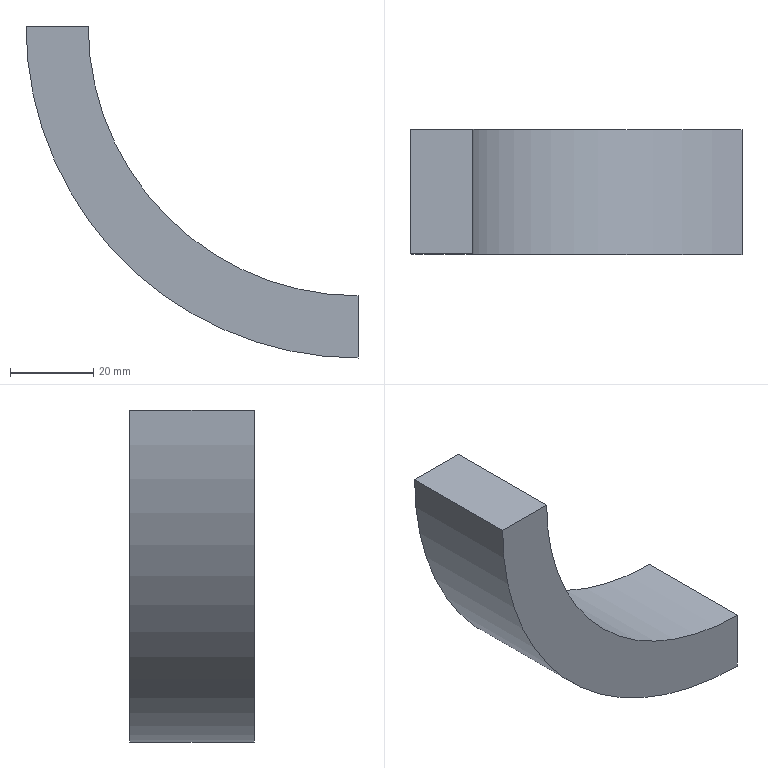Part | SolidWorks | features Extrusion 1 | 1 solid | 6 faces | box 80 x 30 x 80 mm | volume 51247 mm3 | plane 4 | cylinder 2 | commonest cylinder face diameters 130 x1 160 x1
STEP:
#1=CARTESIAN_POINT('',(-65.,0.,0.));
#2=VERTEX_POINT('',#1);
#3=CARTESIAN_POINT('',(0.,0.,-65.));
#4=VERTEX_POINT('',#3);
#5=CARTESIAN_POINT('',(0.,0.,0.));
#6=DIRECTION('',(0.,-1.,0.));
#7=DIRECTION('',(0.,0.,1.));
#8=AXIS2_PLACEMENT_3D('',#5,#6,#7);
#9=CIRCLE('',#8,65.);
#10=EDGE_CURVE('',#2,#4,#9,.T.);
#11=ORIENTED_EDGE('',*,*,#10,.T.);
#12=CARTESIAN_POINT('',(0.,30.,-65.));
#13=VERTEX_POINT('',#12);
#14=CARTESIAN_POINT('',(0.,30.,-65.));
#15=DIRECTION('',(0.,-1.,0.));
#16=VECTOR('',#15,1000.);
#17=LINE('',#14,#16);
#18=EDGE_CURVE('',#13,#4,#17,.T.);
#19=ORIENTED_EDGE('',*,*,#18,.F.);
#20=CARTESIAN_POINT('',(-65.,30.,0.));
#21=VERTEX_POINT('',#20);
#22=CARTESIAN_POINT('',(0.,30.,0.));
#23=DIRECTION('',(0.,-1.,0.));
#24=DIRECTION('',(0.,0.,1.));
#25=AXIS2_PLACEMENT_3D('',#22,#23,#24);
#26=CIRCLE('',#25,65.);
#27=EDGE_CURVE('',#21,#13,#26,.T.);
#28=ORIENTED_EDGE('',*,*,#27,.F.);
#29=CARTESIAN_POINT('',(-65.,30.,0.));
#30=DIRECTION('',(0.,-1.,0.));
#31=VECTOR('',#30,1000.);
#32=LINE('',#29,#31);
#33=EDGE_CURVE('',#21,#2,#32,.T.);
#34=ORIENTED_EDGE('',*,*,#33,.T.);
#35=EDGE_LOOP('',(#11,#19,#28,#34));
#36=FACE_OUTER_BOUND('',#35,.T.);
#37=CARTESIAN_POINT('',(0.,30.,0.));
#38=DIRECTION('',(0.,-1.,0.));
#39=DIRECTION('',(0.,0.,-1.));
#40=AXIS2_PLACEMENT_3D('',#37,#38,#39);
#41=CYLINDRICAL_SURFACE('',#40,65.);
#42=ADVANCED_FACE('',(#36),#41,.F.);
#43=CARTESIAN_POINT('',(0.,0.,-80.));
#44=VERTEX_POINT('',#43);
#45=CARTESIAN_POINT('',(0.,0.,-80.));
#46=DIRECTION('',(0.,0.,-1.));
#47=VECTOR('',#46,1000.);
#48=LINE('',#45,#47);
#49=EDGE_CURVE('',#4,#44,#48,.T.);
#50=ORIENTED_EDGE('',*,*,#49,.T.);
#51=CARTESIAN_POINT('',(0.,30.,-80.));
#52=VERTEX_POINT('',#51);
#53=CARTESIAN_POINT('',(0.,30.,-80.));
#54=DIRECTION('',(0.,-1.,0.));
#55=VECTOR('',#54,1000.);
#56=LINE('',#53,#55);
#57=EDGE_CURVE('',#52,#44,#56,.T.);
#58=ORIENTED_EDGE('',*,*,#57,.F.);
#59=CARTESIAN_POINT('',(0.,30.,-80.));
#60=DIRECTION('',(0.,0.,-1.));
#61=VECTOR('',#60,1000.);
#62=LINE('',#59,#61);
#63=EDGE_CURVE('',#13,#52,#62,.T.);
#64=ORIENTED_EDGE('',*,*,#63,.F.);
#65=ORIENTED_EDGE('',*,*,#18,.T.);
#66=EDGE_LOOP('',(#50,#58,#64,#65));
#67=FACE_OUTER_BOUND('',#66,.T.);
#68=CARTESIAN_POINT('',(0.,30.,-80.));
#69=DIRECTION('',(-1.,0.,0.));
#70=DIRECTION('',(0.,0.,1.));
#71=AXIS2_PLACEMENT_3D('',#68,#69,#70);
#72=PLANE('',#71);
#73=ADVANCED_FACE('',(#67),#72,.F.);
#74=CARTESIAN_POINT('',(-80.,0.,0.));
#75=VERTEX_POINT('',#74);
#76=CARTESIAN_POINT('',(0.,0.,0.));
#77=DIRECTION('',(0.,1.,0.));
#78=DIRECTION('',(0.,0.,1.));
#79=AXIS2_PLACEMENT_3D('',#76,#77,#78);
#80=CIRCLE('',#79,80.);
#81=EDGE_CURVE('',#44,#75,#80,.T.);
#82=ORIENTED_EDGE('',*,*,#81,.T.);
#83=CARTESIAN_POINT('',(-80.,30.,0.));
#84=VERTEX_POINT('',#83);
#85=CARTESIAN_POINT('',(-80.,30.,0.));
#86=DIRECTION('',(0.,-1.,0.));
#87=VECTOR('',#86,1000.);
#88=LINE('',#85,#87);
#89=EDGE_CURVE('',#84,#75,#88,.T.);
#90=ORIENTED_EDGE('',*,*,#89,.F.);
#91=CARTESIAN_POINT('',(0.,30.,0.));
#92=DIRECTION('',(0.,1.,0.));
#93=DIRECTION('',(0.,0.,1.));
#94=AXIS2_PLACEMENT_3D('',#91,#92,#93);
#95=CIRCLE('',#94,80.);
#96=EDGE_CURVE('',#52,#84,#95,.T.);
#97=ORIENTED_EDGE('',*,*,#96,.F.);
#98=ORIENTED_EDGE('',*,*,#57,.T.);
#99=EDGE_LOOP('',(#82,#90,#97,#98));
#100=FACE_OUTER_BOUND('',#99,.T.);
#101=CARTESIAN_POINT('',(0.,30.,0.));
#102=DIRECTION('',(0.,-1.,0.));
#103=DIRECTION('',(0.,0.,-1.));
#104=AXIS2_PLACEMENT_3D('',#101,#102,#103);
#105=CYLINDRICAL_SURFACE('',#104,80.);
#106=ADVANCED_FACE('',(#100),#105,.T.);
#107=CARTESIAN_POINT('',(-80.,0.,0.));
#108=DIRECTION('',(1.,0.,0.));
#109=VECTOR('',#108,1000.);
#110=LINE('',#107,#109);
#111=EDGE_CURVE('',#75,#2,#110,.T.);
#112=ORIENTED_EDGE('',*,*,#111,.T.);
#113=ORIENTED_EDGE('',*,*,#33,.F.);
#114=CARTESIAN_POINT('',(-80.,30.,0.));
#115=DIRECTION('',(1.,0.,0.));
#116=VECTOR('',#115,1000.);
#117=LINE('',#114,#116);
#118=EDGE_CURVE('',#84,#21,#117,.T.);
#119=ORIENTED_EDGE('',*,*,#118,.F.);
#120=ORIENTED_EDGE('',*,*,#89,.T.);
#121=EDGE_LOOP('',(#112,#113,#119,#120));
#122=FACE_OUTER_BOUND('',#121,.T.);
#123=CARTESIAN_POINT('',(-80.,30.,0.));
#124=DIRECTION('',(0.,0.,-1.));
#125=DIRECTION('',(-1.,0.,0.));
#126=AXIS2_PLACEMENT_3D('',#123,#124,#125);
#127=PLANE('',#126);
#128=ADVANCED_FACE('',(#122),#127,.F.);
#129=ORIENTED_EDGE('',*,*,#27,.T.);
#130=ORIENTED_EDGE('',*,*,#63,.T.);
#131=ORIENTED_EDGE('',*,*,#96,.T.);
#132=ORIENTED_EDGE('',*,*,#118,.T.);
#133=EDGE_LOOP('',(#129,#130,#131,#132));
#134=FACE_OUTER_BOUND('',#133,.T.);
#135=CARTESIAN_POINT('',(0.,30.,0.));
#136=DIRECTION('',(0.,1.,0.));
#137=DIRECTION('',(0.,0.,1.));
#138=AXIS2_PLACEMENT_3D('',#135,#136,#137);
#139=PLANE('',#138);
#140=ADVANCED_FACE('',(#134),#139,.T.);
#141=ORIENTED_EDGE('',*,*,#10,.F.);
#142=ORIENTED_EDGE('',*,*,#111,.F.);
#143=ORIENTED_EDGE('',*,*,#81,.F.);
#144=ORIENTED_EDGE('',*,*,#49,.F.);
#145=EDGE_LOOP('',(#141,#142,#143,#144));
#146=FACE_OUTER_BOUND('',#145,.T.);
#147=CARTESIAN_POINT('',(0.,0.,0.));
#148=DIRECTION('',(0.,1.,0.));
#149=DIRECTION('',(0.,0.,1.));
#150=AXIS2_PLACEMENT_3D('',#147,#148,#149);
#151=PLANE('',#150);
#152=ADVANCED_FACE('',(#146),#151,.F.);
#153=CLOSED_SHELL('',(#42,#73,#106,#128,#140,#152));
#154=MANIFOLD_SOLID_BREP('',#153);
#155=CARTESIAN_POINT('',(0.,0.,0.));
#156=DIRECTION('',(0.,0.,1.));
#157=DIRECTION('',(1.,0.,0.));
#158=AXIS2_PLACEMENT_3D('',#155,#156,#157);
#159=(LENGTH_UNIT()NAMED_UNIT(*)SI_UNIT(.MILLI.,.METRE.));
#160=UNCERTAINTY_MEASURE_WITH_UNIT(LENGTH_MEASURE(0.00001),#159,'','');
#161=(NAMED_UNIT(*)PLANE_ANGLE_UNIT()SI_UNIT($,.RADIAN.));
#162=(NAMED_UNIT(*)SI_UNIT($,.STERADIAN.)SOLID_ANGLE_UNIT());
#163=(GEOMETRIC_REPRESENTATION_CONTEXT(3)GLOBAL_UNCERTAINTY_ASSIGNED_CONTEXT((#160))GLOBAL_UNIT_ASSIGNED_CONTEXT((#159,#161,#162))REPRESENTATION_CONTEXT('',''));
#164=ADVANCED_BREP_SHAPE_REPRESENTATION('',(#154,#158),#163);